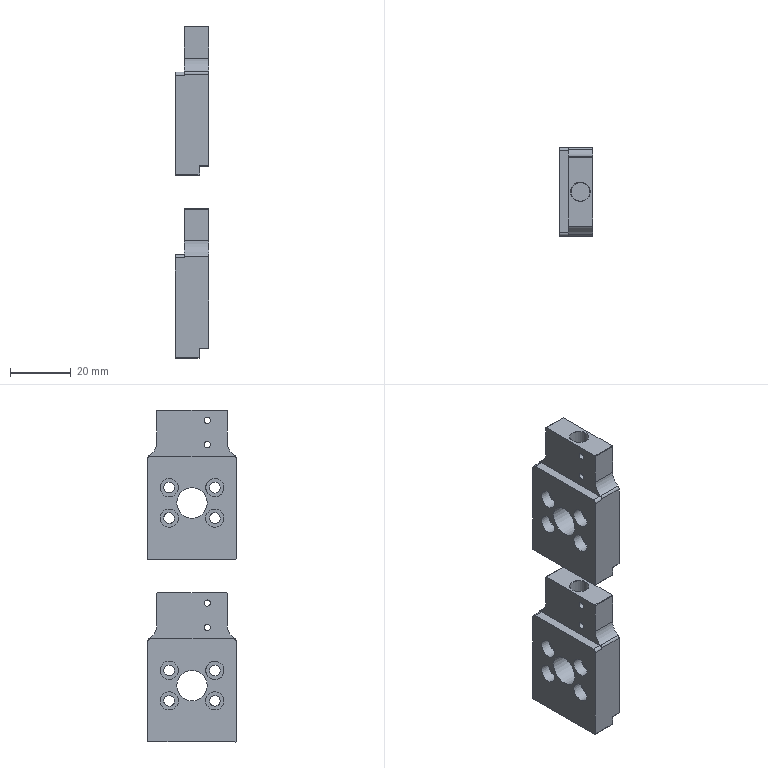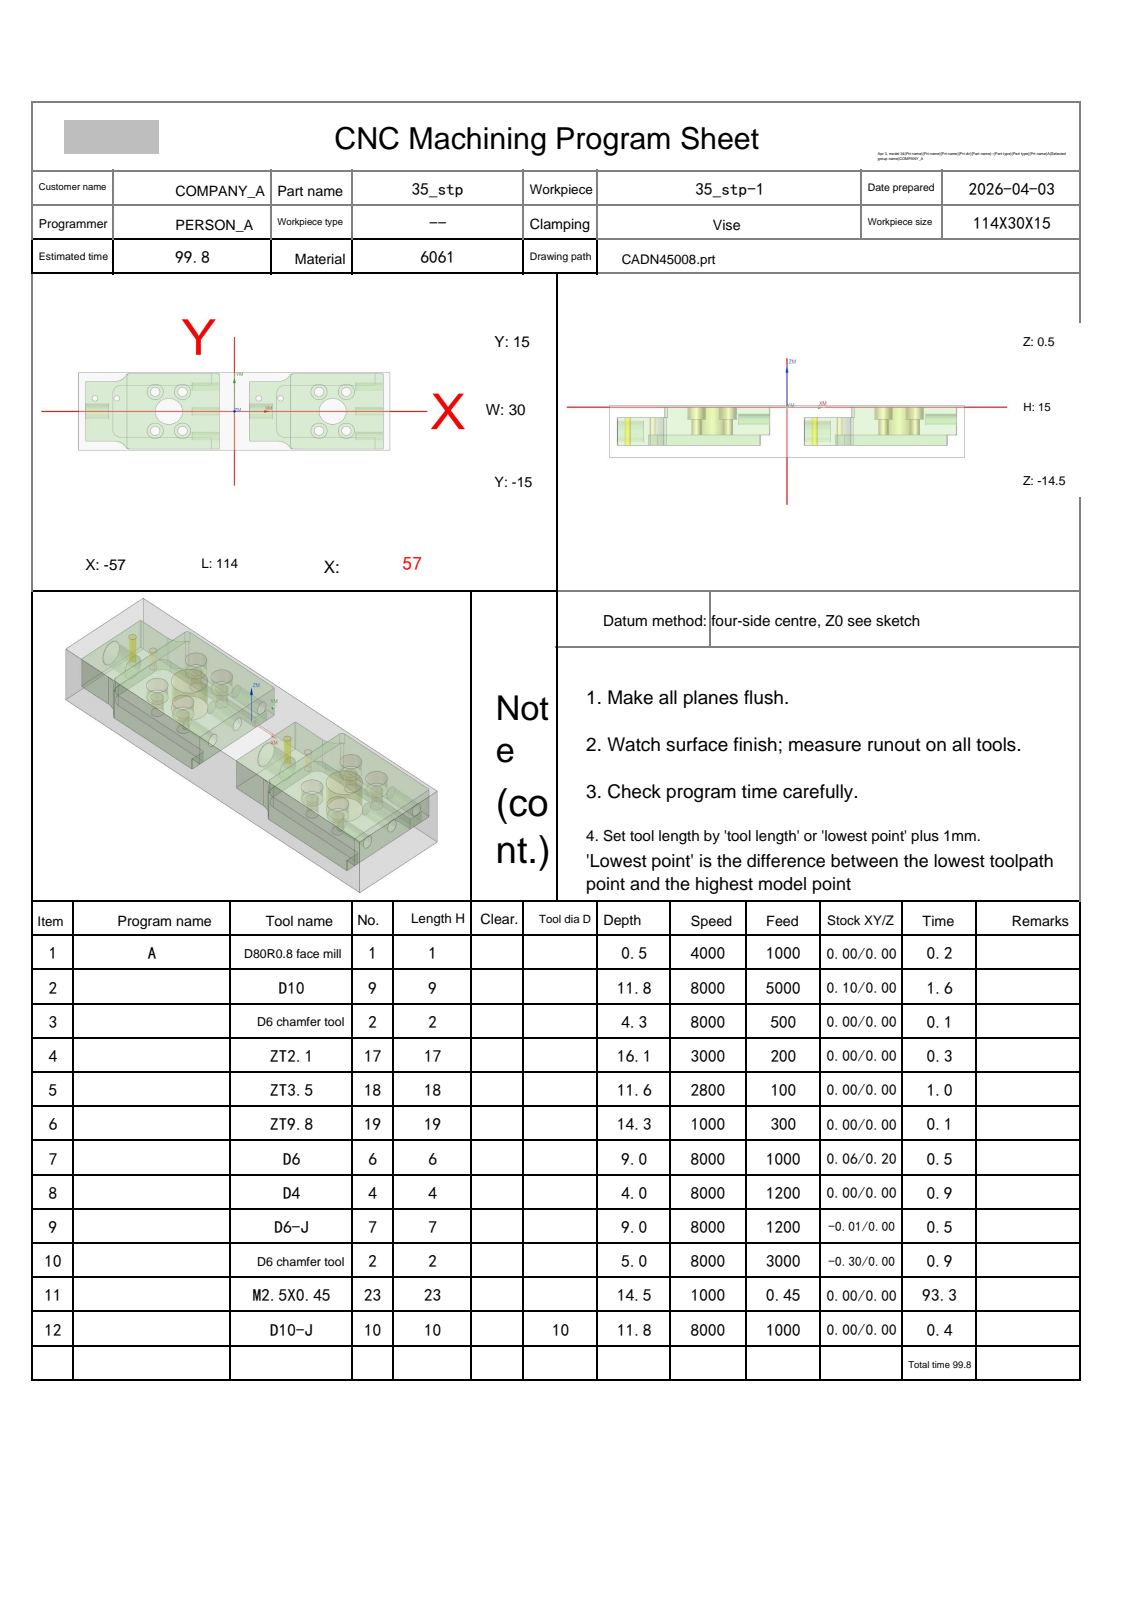NC program | NX | posted by the shop | part box 11 x 29 x 109 mm
Whole program, first 1540 of 2088 lines:
%
O0001
(Machine time: 186.62 MIN)
(===Total Tool:11===)
(T1=D80R0.8 face mill D=80.  R=0.8  D-  H01 Z=0.    )
(T9=D10     D=10.  R=0.   D-  H09 Z=-11.3 )
(T2=D6 chamfer tool   D=6.   R=0.   D-  H02 Z=-4.5  )
(T17=ZT2.1  D=2.1  DR_a=118 D-  H17 Z=-15.63)
(T18=ZT3.5  D=3.5  DR_a=118 D-  H18 Z=-11.05)
(T19=ZT9.8  D=9.8  DR_a=120 D-  H19 Z=-13.83)
(T6=D6      D=6.   R=0.   D-  H06 Z=-8.5  )
(T4=D4      D=4.   R=0.   D4  H04 Z=-3.5  )
(T7=D6-J    D=6.   R=0.   D7  H07 Z=-8.5  )
(T23=M2.5X0.45 D=2.05 DR_a=180 D-  H23 Z=-14.  )
(T10=D10-J  D=10.  R=0.   D10 H10 Z=-11.3 )
G80 G90 G17 G49 G40
G91 G28 Z0
M01
N1 T01 M06
(D80R0.8 face mill  D=80. R=0.8 H=01 ce=0.00 di=0.00)
G00 G90 G54 X99.5 Y0.0 M03 S4000
G43 H01 Z20.
M08
Z2.
G01 Z0.0 F1000.
X94.5
X-94.5
X-99.5
Z2.
G00 Z20.
G91 G28 Z0.0
M05
M09
G91 G28 Z0.0
M01
N2 T09 M06
(D10  D=10. R=0. H=09 ce=0.10 di=0.00)
G00 G90 G54 X-22.118 Y-19.6 M03 S8000
G43 H09 Z20.
M08
Z.5
G01 X-38.736 Z.429 F5000.
G02 X-43.99 Y-16.6 Z.402 I0.0 J6.1
G01 X-54.3 Z.358
G02 X-57.906 Y-15.106 Z.341 I0.0 J5.1
G01 X-58.106 Y-14.906 Z.339
G02 X-59.6 Y-11.3 Z.322 I3.606 J3.606
G01 Y11.3 Z.225
G02 X-58.106 Y14.906 Z.208 I5.1 J0.0
G01 X-57.906 Y15.106 Z.207
G02 X-54.3 Y16.6 Z.19 I3.606 J-3.606
G01 X-43.99 Z.146
G02 X-42.727 Y18.114 Z.137 I5.254 J-3.1
X-38.736 Y19.6 Z.119 I3.99 J-4.614
G01 X-5.7 Z-.023
G02 X-2.094 Y18.106 Z-.04 I0.0 J-5.1
G01 X-1.894 Y17.906 Z-.041
G02 X-.4 Y14.3 Z-.058 I-3.606 J-3.606
G01 Y-14.5 Z-.181
G02 X-5.5 Y-19.6 Z-.216 I-5.1 J0.0
G01 X-38.736 Z-.358
G02 X-43.99 Y-16.6 Z-.385 I0.0 J6.1
G01 X-54.3 Z-.429
G02 X-57.906 Y-15.106 Z-.446 I0.0 J5.1
G01 X-58.106 Y-14.906 Z-.447
G02 X-59.6 Y-11.3 Z-.464 I3.606 J3.606
G01 Y11.3 Z-.561
G02 X-58.106 Y14.906 Z-.578 I5.1 J0.0
G01 X-57.906 Y15.106 Z-.58
G02 X-54.3 Y16.6 Z-.597 I3.606 J-3.606
G01 X-43.99 Z-.641
G02 X-42.727 Y18.114 Z-.649 I5.254 J-3.1
X-38.736 Y19.6 Z-.668 I3.99 J-4.614
G01 X-5.7 Z-.809
G02 X-2.094 Y18.106 Z-.826 I0.0 J-5.1
G01 X-1.894 Y17.906 Z-.828
G02 X-.4 Y14.3 Z-.845 I-3.606 J-3.606
G01 Y-14.5 Z-.968
G02 X-5.5 Y-19.6 Z-1.002 I-5.1 J0.0
G01 X-38.736 Z-1.144
G02 X-43.99 Y-16.6 Z-1.172 I0.0 J6.1
G01 X-54.3 Z-1.216
G02 X-57.906 Y-15.106 Z-1.233 I0.0 J5.1
G01 X-58.106 Y-14.906 Z-1.234
G02 X-59.6 Y-11.3 Z-1.251 I3.606 J3.606
G01 Y11.3 Z-1.348
G02 X-58.106 Y14.906 Z-1.365 I5.1 J0.0
G01 X-57.906 Y15.106 Z-1.366
G02 X-54.3 Y16.6 Z-1.383 I3.606 J-3.606
G01 X-43.99 Z-1.427
G02 X-42.727 Y18.114 Z-1.436 I5.254 J-3.1
X-38.736 Y19.6 Z-1.455 I3.99 J-4.614
G01 X-5.7 Z-1.596
G02 X-2.094 Y18.106 Z-1.613 I0.0 J-5.1
G01 X-1.894 Y17.906 Z-1.614
G02 X-.4 Y14.3 Z-1.631 I-3.606 J-3.606
G01 Y-14.5 Z-1.755
G02 X-5.5 Y-19.6 Z-1.789 I-5.1 J0.0
G01 X-38.736 Z-1.931
G02 X-43.99 Y-16.6 Z-1.958 I0.0 J6.1
G01 X-54.3 Z-2.002
G02 X-57.906 Y-15.106 Z-2.019 I0.0 J5.1
G01 X-58.106 Y-14.906 Z-2.021
G02 X-59.6 Y-11.3 Z-2.038 I3.606 J3.606
G01 Y11.3 Z-2.135
G02 X-58.106 Y14.906 Z-2.152 I5.1 J0.0
G01 X-57.906 Y15.106 Z-2.153
G02 X-54.3 Y16.6 Z-2.17 I3.606 J-3.606
G01 X-43.99 Z-2.214
G02 X-42.727 Y18.114 Z-2.223 I5.254 J-3.1
X-38.736 Y19.6 Z-2.241 I3.99 J-4.614
G01 X-5.7 Z-2.383
G02 X-2.094 Y18.106 Z-2.4 I0.0 J-5.1
G01 X-1.894 Y17.906 Z-2.401
G02 X-.4 Y14.3 Z-2.418 I-3.606 J-3.606
G01 Y-14.5 Z-2.541
G02 X-5.5 Y-19.6 Z-2.576 I-5.1 J0.0
G01 X-38.736 Z-2.718
G02 X-43.99 Y-16.6 Z-2.745 I0.0 J6.1
G01 X-54.3 Z-2.789
G02 X-57.906 Y-15.106 Z-2.806 I0.0 J5.1
G01 X-58.106 Y-14.906 Z-2.807
G02 X-59.6 Y-11.3 Z-2.824 I3.606 J3.606
G01 Y11.3 Z-2.921
G02 X-58.106 Y14.906 Z-2.938 I5.1 J0.0
G01 X-57.906 Y15.106 Z-2.94
G02 X-54.3 Y16.6 Z-2.957 I3.606 J-3.606
G01 X-43.99 Z-3.001
G02 X-42.727 Y18.114 Z-3.009 I5.254 J-3.1
X-38.736 Y19.6 Z-3.028 I3.99 J-4.614
G01 X-5.7 Z-3.169
G02 X-2.094 Y18.106 Z-3.186 I0.0 J-5.1
G01 X-1.894 Y17.906 Z-3.188
G02 X-.4 Y14.3 Z-3.205 I-3.606 J-3.606
G01 Y-14.5 Z-3.328
G02 X-5.5 Y-19.6 Z-3.362 I-5.1 J0.0
G01 X-38.736 Z-3.504
G02 X-43.99 Y-16.6 Z-3.532 I0.0 J6.1
G01 X-54.3 Z-3.576
G02 X-57.906 Y-15.106 Z-3.593 I0.0 J5.1
G01 X-58.106 Y-14.906 Z-3.594
G02 X-59.6 Y-11.3 Z-3.611 I3.606 J3.606
G01 Y11.3 Z-3.708
G02 X-58.106 Y14.906 Z-3.725 I5.1 J0.0
G01 X-57.906 Y15.106 Z-3.726
G02 X-54.3 Y16.6 Z-3.743 I3.606 J-3.606
G01 X-43.99 Z-3.787
G02 X-42.727 Y18.114 Z-3.796 I5.254 J-3.1
X-38.736 Y19.6 Z-3.815 I3.99 J-4.614
G01 X-5.7 Z-3.956
G02 X-2.094 Y18.106 Z-3.973 I0.0 J-5.1
G01 X-1.894 Y17.906 Z-3.974
G02 X-.4 Y14.3 Z-3.991 I-3.606 J-3.606
G01 Y-14.5 Z-4.115
G02 X-5.5 Y-19.6 Z-4.149 I-5.1 J0.0
G01 X-38.736 Z-4.291
G02 X-43.99 Y-16.6 Z-4.318 I0.0 J6.1
G01 X-54.3 Z-4.362
G02 X-57.906 Y-15.106 Z-4.379 I0.0 J5.1
G01 X-58.106 Y-14.906 Z-4.381
G02 X-59.6 Y-11.3 Z-4.398 I3.606 J3.606
G01 Y11.3 Z-4.495
G02 X-58.106 Y14.906 Z-4.512 I5.1 J0.0
G01 X-57.906 Y15.106 Z-4.513
G02 X-54.3 Y16.6 Z-4.53 I3.606 J-3.606
G01 X-43.99 Z-4.574
G02 X-42.727 Y18.114 Z-4.583 I5.254 J-3.1
X-38.736 Y19.6 Z-4.601 I3.99 J-4.614
G01 X-5.7 Z-4.743
G02 X-2.094 Y18.106 Z-4.76 I0.0 J-5.1
G01 X-1.894 Y17.906 Z-4.761
G02 X-.4 Y14.3 Z-4.778 I-3.606 J-3.606
G01 Y-14.5 Z-4.901
G02 X-5.5 Y-19.6 Z-4.936 I-5.1 J0.0
G01 X-38.736 Z-5.078
G02 X-43.99 Y-16.6 Z-5.105 I0.0 J6.1
G01 X-54.3 Z-5.149
G02 X-57.906 Y-15.106 Z-5.166 I0.0 J5.1
G01 X-58.106 Y-14.906 Z-5.167
G02 X-59.6 Y-11.3 Z-5.184 I3.606 J3.606
G01 Y11.3 Z-5.281
G02 X-58.106 Y14.906 Z-5.298 I5.1 J0.0
G01 X-57.906 Y15.106 Z-5.3
G02 X-54.3 Y16.6 Z-5.317 I3.606 J-3.606
G01 X-43.99 Z-5.361
G02 X-42.727 Y18.114 Z-5.369 I5.254 J-3.1
X-38.736 Y19.6 Z-5.388 I3.99 J-4.614
G01 X-5.7 Z-5.529
G02 X-2.094 Y18.106 Z-5.546 I0.0 J-5.1
G01 X-1.894 Y17.906 Z-5.548
G02 X-.4 Y14.3 Z-5.565 I-3.606 J-3.606
G01 Y-14.5 Z-5.688
G02 X-5.5 Y-19.6 Z-5.722 I-5.1 J0.0
G01 X-38.736 Z-5.864
G02 X-43.99 Y-16.6 Z-5.892 I0.0 J6.1
G01 X-54.3 Z-5.936
G02 X-57.906 Y-15.106 Z-5.953 I0.0 J5.1
G01 X-58.106 Y-14.906 Z-5.954
G02 X-59.6 Y-11.3 Z-5.971 I3.606 J3.606
G01 Y11.3 Z-6.068
G02 X-58.106 Y14.906 Z-6.085 I5.1 J0.0
G01 X-57.906 Y15.106 Z-6.086
G02 X-54.3 Y16.6 Z-6.103 I3.606 J-3.606
G01 X-43.99 Z-6.147
G02 X-42.727 Y18.114 Z-6.156 I5.254 J-3.1
X-38.736 Y19.6 Z-6.175 I3.99 J-4.614
G01 X-5.7 Z-6.316
G02 X-2.094 Y18.106 Z-6.333 I0.0 J-5.1
G01 X-1.894 Y17.906 Z-6.334
G02 X-.4 Y14.3 Z-6.351 I-3.606 J-3.606
G01 Y-14.5 Z-6.475
G02 X-5.5 Y-19.6 Z-6.509 I-5.1 J0.0
G01 X-38.736 Z-6.651
G02 X-43.99 Y-16.6 Z-6.678 I0.0 J6.1
G01 X-54.3 Z-6.722
G02 X-57.906 Y-15.106 Z-6.739 I0.0 J5.1
G01 X-58.106 Y-14.906 Z-6.741
G02 X-59.6 Y-11.3 Z-6.758 I3.606 J3.606
G01 Y11.3 Z-6.855
G02 X-58.106 Y14.906 Z-6.872 I5.1 J0.0
G01 X-57.906 Y15.106 Z-6.873
G02 X-54.3 Y16.6 Z-6.89 I3.606 J-3.606
G01 X-43.99 Z-6.934
G02 X-42.727 Y18.114 Z-6.943 I5.254 J-3.1
X-38.736 Y19.6 Z-6.961 I3.99 J-4.614
G01 X-5.7 Z-7.103
G02 X-2.094 Y18.106 Z-7.12 I0.0 J-5.1
G01 X-1.894 Y17.906 Z-7.121
G02 X-.4 Y14.3 Z-7.138 I-3.606 J-3.606
G01 Y-14.5 Z-7.261
G02 X-5.5 Y-19.6 Z-7.296 I-5.1 J0.0
G01 X-38.736 Z-7.438
G02 X-43.99 Y-16.6 Z-7.465 I0.0 J6.1
G01 X-54.3 Z-7.509
G02 X-57.906 Y-15.106 Z-7.526 I0.0 J5.1
G01 X-58.106 Y-14.906 Z-7.527
G02 X-59.6 Y-11.3 Z-7.544 I3.606 J3.606
G01 Y11.3 Z-7.641
G02 X-58.106 Y14.906 Z-7.658 I5.1 J0.0
G01 X-57.906 Y15.106 Z-7.66
G02 X-54.3 Y16.6 Z-7.677 I3.606 J-3.606
G01 X-43.99 Z-7.721
G02 X-42.727 Y18.114 Z-7.729 I5.254 J-3.1
X-38.736 Y19.6 Z-7.748 I3.99 J-4.614
G01 X-5.7 Z-7.889
G02 X-2.094 Y18.106 Z-7.906 I0.0 J-5.1
G01 X-1.894 Y17.906 Z-7.908
G02 X-.4 Y14.3 Z-7.925 I-3.606 J-3.606
G01 Y-14.5 Z-8.048
G02 X-5.5 Y-19.6 Z-8.082 I-5.1 J0.0
G01 X-38.736 Z-8.224
G02 X-43.99 Y-16.6 Z-8.252 I0.0 J6.1
G01 X-54.3 Z-8.296
G02 X-57.906 Y-15.106 Z-8.313 I0.0 J5.1
G01 X-58.106 Y-14.906 Z-8.314
G02 X-59.6 Y-11.3 Z-8.331 I3.606 J3.606
G01 Y11.3 Z-8.428
G02 X-58.106 Y14.906 Z-8.445 I5.1 J0.0
G01 X-57.906 Y15.106 Z-8.446
G02 X-54.3 Y16.6 Z-8.463 I3.606 J-3.606
G01 X-43.99 Z-8.507
G02 X-42.727 Y18.114 Z-8.516 I5.254 J-3.1
X-38.736 Y19.6 Z-8.535 I3.99 J-4.614
G01 X-5.7 Z-8.676
G02 X-2.094 Y18.106 Z-8.693 I0.0 J-5.1
G01 X-1.894 Y17.906 Z-8.694
G02 X-.4 Y14.3 Z-8.711 I-3.606 J-3.606
G01 Y-14.5 Z-8.835
G02 X-5.5 Y-19.6 Z-8.869 I-5.1 J0.0
G01 X-38.736 Z-9.011
G02 X-43.99 Y-16.6 Z-9.038 I0.0 J6.1
G01 X-54.3 Z-9.082
G02 X-57.906 Y-15.106 Z-9.099 I0.0 J5.1
G01 X-58.106 Y-14.906 Z-9.101
G02 X-59.6 Y-11.3 Z-9.118 I3.606 J3.606
G01 Y11.3 Z-9.215
G02 X-58.106 Y14.906 Z-9.232 I5.1 J0.0
G01 X-57.906 Y15.106 Z-9.233
G02 X-54.3 Y16.6 Z-9.25 I3.606 J-3.606
G01 X-43.99 Z-9.294
G02 X-42.727 Y18.114 Z-9.303 I5.254 J-3.1
X-38.736 Y19.6 Z-9.321 I3.99 J-4.614
G01 X-5.7 Z-9.463
G02 X-2.094 Y18.106 Z-9.48 I0.0 J-5.1
G01 X-1.894 Y17.906 Z-9.481
G02 X-.4 Y14.3 Z-9.498 I-3.606 J-3.606
G01 Y-14.5 Z-9.621
G02 X-5.5 Y-19.6 Z-9.656 I-5.1 J0.0
G01 X-38.736 Z-9.798
G02 X-43.99 Y-16.6 Z-9.825 I0.0 J6.1
G01 X-54.3 Z-9.869
G02 X-57.906 Y-15.106 Z-9.886 I0.0 J5.1
G01 X-58.106 Y-14.906 Z-9.887
G02 X-59.6 Y-11.3 Z-9.904 I3.606 J3.606
G01 Y11.3 Z-10.001
G02 X-58.106 Y14.906 Z-10.018 I5.1 J0.0
G01 X-57.906 Y15.106 Z-10.02
G02 X-54.3 Y16.6 Z-10.037 I3.606 J-3.606
G01 X-43.99 Z-10.081
G02 X-42.727 Y18.114 Z-10.089 I5.254 J-3.1
X-38.736 Y19.6 Z-10.108 I3.99 J-4.614
G01 X-5.7 Z-10.249
G02 X-2.094 Y18.106 Z-10.266 I0.0 J-5.1
G01 X-1.894 Y17.906 Z-10.268
G02 X-.4 Y14.3 Z-10.285 I-3.606 J-3.606
G01 Y-14.5 Z-10.408
G02 X-5.5 Y-19.6 Z-10.442 I-5.1 J0.0
G01 X-38.736 Z-10.584
G02 X-43.99 Y-16.6 Z-10.612 I0.0 J6.1
G01 X-54.3 Z-10.656
G02 X-57.906 Y-15.106 Z-10.673 I0.0 J5.1
G01 X-58.106 Y-14.906 Z-10.674
G02 X-59.6 Y-11.3 Z-10.691 I3.606 J3.606
G01 Y11.3 Z-10.788
G02 X-58.106 Y14.906 Z-10.805 I5.1 J0.0
G01 X-57.906 Y15.106 Z-10.806
G02 X-54.3 Y16.6 Z-10.823 I3.606 J-3.606
G01 X-43.99 Z-10.867
G02 X-42.727 Y18.114 Z-10.876 I5.254 J-3.1
X-38.736 Y19.6 Z-10.895 I3.99 J-4.614
G01 X-5.7 Z-11.036
G02 X-2.094 Y18.106 Z-11.053 I0.0 J-5.1
G01 X-1.894 Y17.906 Z-11.054
G02 X-.4 Y14.3 Z-11.071 I-3.606 J-3.606
G01 Y-14.5 Z-11.195
G02 X-5.5 Y-19.6 Z-11.229 I-5.1 J0.0
G01 X-22.118 Z-11.3
X-38.736
G02 X-43.99 Y-16.6 I0.0 J6.1
G01 X-54.3
G02 X-57.906 Y-15.106 I0.0 J5.1
G01 X-58.106 Y-14.906
G02 X-59.6 Y-11.3 I3.606 J3.606
G01 Y11.3
G02 X-58.106 Y14.906 I5.1 J0.0
G01 X-57.906 Y15.106
G02 X-54.3 Y16.6 I3.606 J-3.606
G01 X-43.99
G02 X-38.736 Y19.6 I5.254 J-3.1
G01 X-5.7
G02 X-2.094 Y18.106 I0.0 J-5.1
G01 X-1.894 Y17.906
G02 X-.4 Y14.3 I-3.606 J-3.606
G01 Y-14.5
G02 X-5.5 Y-19.6 I-5.1 J0.0
G01 X-22.118
X-22.618
Z-10.3
G00 Z20.
X37.882
Z.5
G01 X21.264 Z.429
G02 X16.01 Y-16.6 Z.402 I0.0 J6.1
G01 X5.7 Z.358
G02 X2.094 Y-15.106 Z.341 I0.0 J5.1
G01 X1.894 Y-14.906 Z.339
G02 X.4 Y-11.3 Z.322 I3.606 J3.606
G01 Y11.3 Z.225
G02 X1.894 Y14.906 Z.208 I5.1 J0.0
G01 X2.094 Y15.106 Z.207
G02 X5.7 Y16.6 Z.19 I3.606 J-3.606
G01 X16.01 Z.146
G02 X21.264 Y19.6 Z.119 I5.254 J-3.1
G01 X54.3 Z-.023
G02 X57.906 Y18.106 Z-.04 I0.0 J-5.1
G01 X58.106 Y17.906 Z-.041
G02 X59.6 Y14.3 Z-.058 I-3.606 J-3.606
G01 Y-14.5 Z-.181
G02 X54.5 Y-19.6 Z-.216 I-5.1 J0.0
G01 X21.264 Z-.358
G02 X16.01 Y-16.6 Z-.385 I0.0 J6.1
G01 X5.7 Z-.429
G02 X2.094 Y-15.106 Z-.446 I0.0 J5.1
G01 X1.894 Y-14.906 Z-.447
G02 X.4 Y-11.3 Z-.464 I3.606 J3.606
G01 Y11.3 Z-.561
G02 X1.894 Y14.906 Z-.578 I5.1 J0.0
G01 X2.094 Y15.106 Z-.58
G02 X5.7 Y16.6 Z-.597 I3.606 J-3.606
G01 X16.01 Z-.641
G02 X21.264 Y19.6 Z-.668 I5.254 J-3.1
G01 X54.3 Z-.809
G02 X57.906 Y18.106 Z-.826 I0.0 J-5.1
G01 X58.106 Y17.906 Z-.828
G02 X59.6 Y14.3 Z-.845 I-3.606 J-3.606
G01 Y-14.5 Z-.968
G02 X54.5 Y-19.6 Z-1.002 I-5.1 J0.0
G01 X21.264 Z-1.144
G02 X16.01 Y-16.6 Z-1.172 I0.0 J6.1
G01 X5.7 Z-1.216
G02 X2.094 Y-15.106 Z-1.233 I0.0 J5.1
G01 X1.894 Y-14.906 Z-1.234
G02 X.4 Y-11.3 Z-1.251 I3.606 J3.606
G01 Y11.3 Z-1.348
G02 X1.894 Y14.906 Z-1.365 I5.1 J0.0
G01 X2.094 Y15.106 Z-1.366
G02 X5.7 Y16.6 Z-1.383 I3.606 J-3.606
G01 X16.01 Z-1.427
G02 X21.264 Y19.6 Z-1.455 I5.254 J-3.1
G01 X54.3 Z-1.596
G02 X57.906 Y18.106 Z-1.613 I0.0 J-5.1
G01 X58.106 Y17.906 Z-1.614
G02 X59.6 Y14.3 Z-1.631 I-3.606 J-3.606
G01 Y-14.5 Z-1.755
G02 X54.5 Y-19.6 Z-1.789 I-5.1 J0.0
G01 X21.264 Z-1.931
G02 X16.01 Y-16.6 Z-1.958 I0.0 J6.1
G01 X5.7 Z-2.002
G02 X2.094 Y-15.106 Z-2.019 I0.0 J5.1
G01 X1.894 Y-14.906 Z-2.021
G02 X.4 Y-11.3 Z-2.038 I3.606 J3.606
G01 Y11.3 Z-2.135
G02 X1.894 Y14.906 Z-2.152 I5.1 J0.0
G01 X2.094 Y15.106 Z-2.153
G02 X5.7 Y16.6 Z-2.17 I3.606 J-3.606
G01 X16.01 Z-2.214
G02 X21.264 Y19.6 Z-2.241 I5.254 J-3.1
G01 X54.3 Z-2.383
G02 X57.906 Y18.106 Z-2.4 I0.0 J-5.1
G01 X58.106 Y17.906 Z-2.401
G02 X59.6 Y14.3 Z-2.418 I-3.606 J-3.606
G01 Y-14.5 Z-2.541
G02 X54.5 Y-19.6 Z-2.576 I-5.1 J0.0
G01 X21.264 Z-2.718
G02 X16.01 Y-16.6 Z-2.745 I0.0 J6.1
G01 X5.7 Z-2.789
G02 X2.094 Y-15.106 Z-2.806 I0.0 J5.1
G01 X1.894 Y-14.906 Z-2.807
G02 X.4 Y-11.3 Z-2.824 I3.606 J3.606
G01 Y11.3 Z-2.921
G02 X1.894 Y14.906 Z-2.938 I5.1 J0.0
G01 X2.094 Y15.106 Z-2.94
G02 X5.7 Y16.6 Z-2.957 I3.606 J-3.606
G01 X16.01 Z-3.001
G02 X21.264 Y19.6 Z-3.028 I5.254 J-3.1
G01 X54.3 Z-3.169
G02 X57.906 Y18.106 Z-3.186 I0.0 J-5.1
G01 X58.106 Y17.906 Z-3.188
G02 X59.6 Y14.3 Z-3.205 I-3.606 J-3.606
G01 Y-14.5 Z-3.328
G02 X54.5 Y-19.6 Z-3.362 I-5.1 J0.0
G01 X21.264 Z-3.504
G02 X16.01 Y-16.6 Z-3.532 I0.0 J6.1
G01 X5.7 Z-3.576
G02 X2.094 Y-15.106 Z-3.593 I0.0 J5.1
G01 X1.894 Y-14.906 Z-3.594
G02 X.4 Y-11.3 Z-3.611 I3.606 J3.606
G01 Y11.3 Z-3.708
G02 X1.894 Y14.906 Z-3.725 I5.1 J0.0
G01 X2.094 Y15.106 Z-3.726
G02 X5.7 Y16.6 Z-3.743 I3.606 J-3.606
G01 X16.01 Z-3.787
G02 X21.264 Y19.6 Z-3.815 I5.254 J-3.1
G01 X54.3 Z-3.956
G02 X57.906 Y18.106 Z-3.973 I0.0 J-5.1
G01 X58.106 Y17.906 Z-3.974
G02 X59.6 Y14.3 Z-3.991 I-3.606 J-3.606
G01 Y-14.5 Z-4.115
G02 X54.5 Y-19.6 Z-4.149 I-5.1 J0.0
G01 X21.264 Z-4.291
G02 X16.01 Y-16.6 Z-4.318 I0.0 J6.1
G01 X5.7 Z-4.362
G02 X2.094 Y-15.106 Z-4.379 I0.0 J5.1
G01 X1.894 Y-14.906 Z-4.381
G02 X.4 Y-11.3 Z-4.398 I3.606 J3.606
G01 Y11.3 Z-4.495
G02 X1.894 Y14.906 Z-4.512 I5.1 J0.0
G01 X2.094 Y15.106 Z-4.513
G02 X5.7 Y16.6 Z-4.53 I3.606 J-3.606
G01 X16.01 Z-4.574
G02 X21.264 Y19.6 Z-4.601 I5.254 J-3.1
G01 X54.3 Z-4.743
G02 X57.906 Y18.106 Z-4.76 I0.0 J-5.1
G01 X58.106 Y17.906 Z-4.761
G02 X59.6 Y14.3 Z-4.778 I-3.606 J-3.606
G01 Y-14.5 Z-4.901
G02 X54.5 Y-19.6 Z-4.936 I-5.1 J0.0
G01 X21.264 Z-5.078
G02 X16.01 Y-16.6 Z-5.105 I0.0 J6.1
G01 X5.7 Z-5.149
G02 X2.094 Y-15.106 Z-5.166 I0.0 J5.1
G01 X1.894 Y-14.906 Z-5.167
G02 X.4 Y-11.3 Z-5.184 I3.606 J3.606
G01 Y11.3 Z-5.281
G02 X1.894 Y14.906 Z-5.298 I5.1 J0.0
G01 X2.094 Y15.106 Z-5.3
G02 X5.7 Y16.6 Z-5.317 I3.606 J-3.606
G01 X16.01 Z-5.361
G02 X21.264 Y19.6 Z-5.388 I5.254 J-3.1
G01 X54.3 Z-5.529
G02 X57.906 Y18.106 Z-5.546 I0.0 J-5.1
G01 X58.106 Y17.906 Z-5.548
G02 X59.6 Y14.3 Z-5.565 I-3.606 J-3.606
G01 Y-14.5 Z-5.688
G02 X54.5 Y-19.6 Z-5.722 I-5.1 J0.0
G01 X21.264 Z-5.864
G02 X16.01 Y-16.6 Z-5.892 I0.0 J6.1
G01 X5.7 Z-5.936
G02 X2.094 Y-15.106 Z-5.953 I0.0 J5.1
G01 X1.894 Y-14.906 Z-5.954
G02 X.4 Y-11.3 Z-5.971 I3.606 J3.606
G01 Y11.3 Z-6.068
G02 X1.894 Y14.906 Z-6.085 I5.1 J0.0
G01 X2.094 Y15.106 Z-6.086
G02 X5.7 Y16.6 Z-6.103 I3.606 J-3.606
G01 X16.01 Z-6.147
G02 X21.264 Y19.6 Z-6.175 I5.254 J-3.1
G01 X54.3 Z-6.316
G02 X57.906 Y18.106 Z-6.333 I0.0 J-5.1
G01 X58.106 Y17.906 Z-6.334
G02 X59.6 Y14.3 Z-6.351 I-3.606 J-3.606
G01 Y-14.5 Z-6.475
G02 X54.5 Y-19.6 Z-6.509 I-5.1 J0.0
G01 X21.264 Z-6.651
G02 X16.01 Y-16.6 Z-6.678 I0.0 J6.1
G01 X5.7 Z-6.722
G02 X2.094 Y-15.106 Z-6.739 I0.0 J5.1
G01 X1.894 Y-14.906 Z-6.741
G02 X.4 Y-11.3 Z-6.758 I3.606 J3.606
G01 Y11.3 Z-6.855
G02 X1.894 Y14.906 Z-6.872 I5.1 J0.0
G01 X2.094 Y15.106 Z-6.873
G02 X5.7 Y16.6 Z-6.89 I3.606 J-3.606
G01 X16.01 Z-6.934
G02 X21.264 Y19.6 Z-6.961 I5.254 J-3.1
G01 X54.3 Z-7.103
G02 X57.906 Y18.106 Z-7.12 I0.0 J-5.1
G01 X58.106 Y17.906 Z-7.121
G02 X59.6 Y14.3 Z-7.138 I-3.606 J-3.606
G01 Y-14.5 Z-7.261
G02 X54.5 Y-19.6 Z-7.296 I-5.1 J0.0
G01 X21.264 Z-7.438
G02 X16.01 Y-16.6 Z-7.465 I0.0 J6.1
G01 X5.7 Z-7.509
G02 X2.094 Y-15.106 Z-7.526 I0.0 J5.1
G01 X1.894 Y-14.906 Z-7.527
G02 X.4 Y-11.3 Z-7.544 I3.606 J3.606
G01 Y11.3 Z-7.641
G02 X1.894 Y14.906 Z-7.658 I5.1 J0.0
G01 X2.094 Y15.106 Z-7.66
G02 X5.7 Y16.6 Z-7.677 I3.606 J-3.606
G01 X16.01 Z-7.721
G02 X21.264 Y19.6 Z-7.748 I5.254 J-3.1
G01 X54.3 Z-7.889
G02 X57.906 Y18.106 Z-7.906 I0.0 J-5.1
G01 X58.106 Y17.906 Z-7.908
G02 X59.6 Y14.3 Z-7.925 I-3.606 J-3.606
G01 Y-14.5 Z-8.048
G02 X54.5 Y-19.6 Z-8.082 I-5.1 J0.0
G01 X21.264 Z-8.224
G02 X16.01 Y-16.6 Z-8.252 I0.0 J6.1
G01 X5.7 Z-8.296
G02 X2.094 Y-15.106 Z-8.313 I0.0 J5.1
G01 X1.894 Y-14.906 Z-8.314
G02 X.4 Y-11.3 Z-8.331 I3.606 J3.606
G01 Y11.3 Z-8.428
G02 X1.894 Y14.906 Z-8.445 I5.1 J0.0
G01 X2.094 Y15.106 Z-8.446
G02 X5.7 Y16.6 Z-8.463 I3.606 J-3.606
G01 X16.01 Z-8.507
G02 X21.264 Y19.6 Z-8.535 I5.254 J-3.1
G01 X54.3 Z-8.676
G02 X57.906 Y18.106 Z-8.693 I0.0 J-5.1
G01 X58.106 Y17.906 Z-8.694
G02 X59.6 Y14.3 Z-8.711 I-3.606 J-3.606
G01 Y-14.5 Z-8.835
G02 X54.5 Y-19.6 Z-8.869 I-5.1 J0.0
G01 X21.264 Z-9.011
G02 X16.01 Y-16.6 Z-9.038 I0.0 J6.1
G01 X5.7 Z-9.082
G02 X2.094 Y-15.106 Z-9.099 I0.0 J5.1
G01 X1.894 Y-14.906 Z-9.101
G02 X.4 Y-11.3 Z-9.118 I3.606 J3.606
G01 Y11.3 Z-9.215
G02 X1.894 Y14.906 Z-9.232 I5.1 J0.0
G01 X2.094 Y15.106 Z-9.233
G02 X5.7 Y16.6 Z-9.25 I3.606 J-3.606
G01 X16.01 Z-9.294
G02 X21.264 Y19.6 Z-9.321 I5.254 J-3.1
G01 X54.3 Z-9.463
G02 X57.906 Y18.106 Z-9.48 I0.0 J-5.1
G01 X58.106 Y17.906 Z-9.481
G02 X59.6 Y14.3 Z-9.498 I-3.606 J-3.606
G01 Y-14.5 Z-9.621
G02 X54.5 Y-19.6 Z-9.656 I-5.1 J0.0
G01 X21.264 Z-9.798
G02 X16.01 Y-16.6 Z-9.825 I0.0 J6.1
G01 X5.7 Z-9.869
G02 X2.094 Y-15.106 Z-9.886 I0.0 J5.1
G01 X1.894 Y-14.906 Z-9.887
G02 X.4 Y-11.3 Z-9.904 I3.606 J3.606
G01 Y11.3 Z-10.001
G02 X1.894 Y14.906 Z-10.018 I5.1 J0.0
G01 X2.094 Y15.106 Z-10.02
G02 X5.7 Y16.6 Z-10.037 I3.606 J-3.606
G01 X16.01 Z-10.081
G02 X21.264 Y19.6 Z-10.108 I5.254 J-3.1
G01 X54.3 Z-10.249
G02 X57.906 Y18.106 Z-10.266 I0.0 J-5.1
G01 X58.106 Y17.906 Z-10.268
G02 X59.6 Y14.3 Z-10.285 I-3.606 J-3.606
G01 Y-14.5 Z-10.408
G02 X54.5 Y-19.6 Z-10.442 I-5.1 J0.0
G01 X21.264 Z-10.584
G02 X16.01 Y-16.6 Z-10.612 I0.0 J6.1
G01 X5.7 Z-10.656
G02 X2.094 Y-15.106 Z-10.673 I0.0 J5.1
G01 X1.894 Y-14.906 Z-10.674
G02 X.4 Y-11.3 Z-10.691 I3.606 J3.606
G01 Y11.3 Z-10.788
G02 X1.894 Y14.906 Z-10.805 I5.1 J0.0
G01 X2.094 Y15.106 Z-10.806
G02 X5.7 Y16.6 Z-10.823 I3.606 J-3.606
G01 X16.01 Z-10.867
G02 X21.264 Y19.6 Z-10.895 I5.254 J-3.1
G01 X54.3 Z-11.036
G02 X57.906 Y18.106 Z-11.053 I0.0 J-5.1
G01 X58.106 Y17.906 Z-11.054
G02 X59.6 Y14.3 Z-11.071 I-3.606 J-3.606
G01 Y-14.5 Z-11.195
G02 X54.5 Y-19.6 Z-11.229 I-5.1 J0.0
G01 X37.882 Z-11.3
X21.264
G02 X16.01 Y-16.6 I0.0 J6.1
G01 X5.7
G02 X2.094 Y-15.106 I0.0 J5.1
G01 X1.894 Y-14.906
G02 X.4 Y-11.3 I3.606 J3.606
G01 Y11.3
G02 X1.894 Y14.906 I5.1 J0.0
G01 X2.094 Y15.106
G02 X5.7 Y16.6 I3.606 J-3.606
G01 X16.01
G02 X21.264 Y19.6 I5.254 J-3.1
G01 X54.3
G02 X57.906 Y18.106 I0.0 J-5.1
G01 X58.106 Y17.906
G02 X59.6 Y14.3 I-3.606 J-3.606
G01 Y-14.5
G02 X54.5 Y-19.6 I-5.1 J0.0
G01 X37.882
X37.382
Z-10.3
G00 Z20.
G00 G90 X10.025 Y-19.5 M03 S6000
Z20.
Z.017
G01 Z-.483 F3500.
Y-8.
X11.05
Y8.
X9.
Y-8.
X10.025
Y-12.5
X15.55
Y12.5
X5.286
X4.5 Y11.714
Y-11.714
X5.286 Y-12.5
X10.025
X10.525
Z.017
G00 Z.5
X10.025 Y-19.5
Z-.467
G01 Z-.967
Y-8.
X11.05
Y8.
X9.
Y-8.
X10.025
Y-12.5
X15.55
Y12.5
X5.286
X4.5 Y11.714
Y-11.714
X5.286 Y-12.5
X10.025
X10.525
Z-.467
G00 Z.017
X10.025 Y-19.5
Z-.95
G01 Z-1.45
Y-8.
X11.05
Y8.
X9.
Y-8.
X10.025
Y-12.5
X15.55
Y12.5
X5.286
X4.5 Y11.714
Y-11.714
X5.286 Y-12.5
X10.025
X10.525
Z-.95
G00 Z-.467
X10.025 Y-19.5
Z-1.433
G01 Z-1.933
Y-8.
X11.05
Y8.
X9.
Y-8.
X10.025
Y-12.5
X15.55
Y12.5
X5.286
X4.5 Y11.714
Y-11.714
X5.286 Y-12.5
X10.025
X10.525
Z-1.433
G00 Z-.95
X10.025 Y-19.5
Z-1.917
G01 Z-2.417
Y-8.
X11.05
Y8.
X9.
Y-8.
X10.025
Y-12.5
X15.55
Y12.5
X5.286
X4.5 Y11.714
Y-11.714
X5.286 Y-12.5
X10.025
X10.525
Z-1.917
G00 Z-1.433
X10.025 Y-19.5
Z-2.4
G01 Z-2.9
Y-8.
X11.05
Y8.
X9.
Y-8.
X10.025
Y-12.5
X15.55
Y12.5
X5.286
X4.5 Y11.714
Y-11.714
X5.286 Y-12.5
X10.025
X10.525
Z-2.4
G00 Z20.
X-62.5 Y0.0
Z.017
G01 Z-.483
X-51.
Y-8.
X-48.95
Y8.
X-51.
Y0.0
X-55.5
Y-11.714
X-54.714 Y-12.5
X-44.45
Y12.5
X-54.714
X-55.5 Y11.714
Y0.0
Y-.5
Z.017
G00 Z.5
X-62.5 Y0.0
Z-.467
G01 Z-.967
X-51.
Y-8.
X-48.95
Y8.
X-51.
Y0.0
X-55.5
Y-11.714
X-54.714 Y-12.5
X-44.45
Y12.5
X-54.714
X-55.5 Y11.714
Y0.0
Y-.5
Z-.467
G00 Z.017
X-62.5 Y0.0
Z-.95
G01 Z-1.45
X-51.
Y-8.
X-48.95
Y8.
X-51.
Y0.0
X-55.5
Y-11.714
X-54.714 Y-12.5
X-44.45
Y12.5
X-54.714
X-55.5 Y11.714
Y0.0
Y-.5
Z-.95
G00 Z-.467
X-62.5 Y0.0
Z-1.433
G01 Z-1.933
X-51.
Y-8.
X-48.95
Y8.
X-51.
Y0.0
X-55.5
Y-11.714
X-54.714 Y-12.5
X-44.45
Y12.5
X-54.714
X-55.5 Y11.714
Y0.0
Y-.5
Z-1.433
G00 Z-.95
X-62.5 Y0.0
Z-1.917
G01 Z-2.417
X-51.
Y-8.
X-48.95
Y8.
X-51.
Y0.0
X-55.5
Y-11.714
X-54.714 Y-12.5
X-44.45
Y12.5
X-54.714
X-55.5 Y11.714
Y0.0
Y-.5
Z-1.917
G00 Z-1.433
X-62.5 Y0.0
Z-2.4
G01 Z-2.9
X-51.
Y-8.
X-48.95
Y8.
X-51.
Y0.0
X-55.5
Y-11.714
X-54.714 Y-12.5
X-44.45
Y12.5
X-54.714
X-55.5 Y11.714
Y0.0
Y-.5
Z-2.4
G00 Z20.
G91 G28 Z0.0
M05
M09
G91 G28 Z0.0
M01
N3 T02 M06
(D6 chamfer tool  D=6. R=0. H=02 ce=0.00 di=0.10)
G00 G90 G54 X-51.1 Y5. M03 S8000
G43 H02 Z20.
M08
G98 G81 X-51.1 Y5. Z-3.8 R-2. F500.
X-43.1
X-29. Y7.5 Z-.8 R1.
X-19.
X-24. Y0.0
X-29. Y-7.5
X-19.
X8.9 Y5. Z-3.8 R-2.
X16.9
X31. Y7.5 Z-.8 R1.
X41.
X36. Y0.0
X41. Y-7.5
X31.
G80
G00 Z20.
G00 G90 X-51.1 Y5. M03 S8000
Z20.
G98 G81 X-51.1 Y5. Z-3.8 R-2. F500.
X-43.1
X8.9
X16.9
G80
G00 Z20.
G91 G28 Z0.0
M05
M09
G91 G28 Z0.0
M01
N4 T17 M06
(ZT2.1 D=2.1 DR_a=118 H=17)
G00 G90 G54 X-51.1 Y5. M03 S3000
G43 H17 Z20.
M08
G98 G83 X-51.1 Y5. Z-15.631 R-2. F200. Q2.
G98 G83 X-43.1 Y5. Z-12.631 R-2. Q2.
G98 G83 X8.9 Y5. Z-15.631 R-2. Q2.
G98 G83 X16.9 Y5. Z-12.631 R-2. Q2.
G80
G00 Z20.
G91 G28 Z0.0
M05
M09
G91 G28 Z0.0
M01
N5 T18 M06
(ZT3.5 D=3.5 DR_a=118 H=18)
G00 G90 G54 X-19. Y7.5 M03 S2800
G43 H18 Z20.
M08
G98 G83 X-19. Y7.5 Z-11.052 R1. F100. Q2.
X-29.
Y-7.5
X-19.
X31.
X41.
Y7.5
X31.
G80
G00 Z20.
G91 G28 Z0.0
M05
M09
G91 G28 Z0.0
M01
N6 T19 M06
(ZT9.8 D=9.8 DR_a=120 H=19)
G00 G90 G54 X-24. Y0.0 M03 S1000
G43 H19 Z20.
M08
G98 G83 X-24. Y0.0 Z-13.829 R1. F300. Q2.
X36.
G80
G00 Z20.
G91 G28 Z0.0
M05
M09
G91 G28 Z0.0
M01
N7 T06 M06
(D6  D=6. R=0. H=06 ce=0.06 di=0.20)
G00 G90 G54 X-24. Y0.0 M03 S8000
G43 H06 Z20.
M08
Z.5
G03 X-24.97 Y-.97 I0.0 J-.97 F1000.
X-24. Y-1.94 I.97 J0.0
X-24. Y-1.94 Z0.0 I0.0 J1.94
X-24. Y-1.94 Z-.5 I0.0 J1.94
X-24. Y-1.94 Z-1. I0.0 J1.94
X-24. Y-1.94 Z-1.5 I0.0 J1.94
X-24. Y-1.94 Z-2. I0.0 J1.94
X-24. Y-1.94 Z-2.5 I0.0 J1.94
X-24. Y-1.94 Z-3. I0.0 J1.94
X-24. Y-1.94 Z-3.5 I0.0 J1.94
X-24. Y-1.94 Z-4. I0.0 J1.94
X-24. Y-1.94 Z-4.5 I0.0 J1.94
X-24. Y-1.94 Z-5. I0.0 J1.94
X-24. Y-1.94 Z-5.5 I0.0 J1.94
X-24. Y-1.94 Z-6. I0.0 J1.94
X-24. Y-1.94 Z-6.5 I0.0 J1.94
X-24. Y-1.94 Z-7. I0.0 J1.94
X-24. Y-1.94 Z-7.5 I0.0 J1.94
X-24. Y-1.94 Z-8. I0.0 J1.94
X-24. Y-1.94 Z-8.5 I0.0 J1.94
X-22.06 Y0.0 I0.0 J1.94
X-24. Y1.94 I-1.94 J0.0
X-25.94 Y0.0 I0.0 J-1.94
X-24. Y-1.94 I1.94 J0.0
X-23.03 Y-.97 I0.0 J.97
X-24. Y0.0 I-.97 J0.0
G00 Z20.
X36.
Z.5
G03 X35.03 Y-.97 I0.0 J-.97
X36. Y-1.94 I.97 J0.0
X36. Y-1.94 Z0.0 I0.0 J1.94
X36. Y-1.94 Z-.5 I0.0 J1.94
X36. Y-1.94 Z-1. I0.0 J1.94
X36. Y-1.94 Z-1.5 I0.0 J1.94
X36. Y-1.94 Z-2. I0.0 J1.94
X36. Y-1.94 Z-2.5 I0.0 J1.94
X36. Y-1.94 Z-3. I0.0 J1.94
X36. Y-1.94 Z-3.5 I0.0 J1.94
X36. Y-1.94 Z-4. I0.0 J1.94
X36. Y-1.94 Z-4.5 I0.0 J1.94
X36. Y-1.94 Z-5. I0.0 J1.94
X36. Y-1.94 Z-5.5 I0.0 J1.94
X36. Y-1.94 Z-6. I0.0 J1.94
X36. Y-1.94 Z-6.5 I0.0 J1.94
X36. Y-1.94 Z-7. I0.0 J1.94
X36. Y-1.94 Z-7.5 I0.0 J1.94
X36. Y-1.94 Z-8. I0.0 J1.94
X36. Y-1.94 Z-8.5 I0.0 J1.94
X37.94 Y0.0 I0.0 J1.94
X36. Y1.94 I-1.94 J0.0
X34.06 Y0.0 I0.0 J-1.94
X36. Y-1.94 I1.94 J0.0
X36.97 Y-.97 I0.0 J.97
X36. Y0.0 I-.97 J0.0
G00 Z20.
G91 G28 Z0.0
M05
M09
G91 G28 Z0.0
M01
N8 T04 M06
(D4  D=4. R=0. H=04 ce=0.10 di=0.00)
G00 G90 G54 X-19. Y-7.5 M03 S8000
G43 H04 Z20.
M08
Z.5
G03 X-19.45 Y-7.95 I0.0 J-.45 F1200.
X-19. Y-8.4 I.45 J0.0
X-19. Y-8.4 Z.2 I0.0 J.9
X-19. Y-8.4 Z-.1 I0.0 J.9
X-19. Y-8.4 Z-.4 I0.0 J.9
X-19. Y-8.4 Z-.7 I0.0 J.9
X-19. Y-8.4 Z-1. I0.0 J.9
X-19. Y-8.4 Z-1.3 I0.0 J.9
X-19. Y-8.4 Z-1.6 I0.0 J.9
X-19. Y-8.4 Z-1.9 I0.0 J.9
X-19. Y-8.4 Z-2.2 I0.0 J.9
X-19. Y-8.4 Z-2.5 I0.0 J.9
X-19. Y-8.4 Z-2.8 I0.0 J.9
X-19. Y-8.4 Z-3.1 I0.0 J.9
X-19. Y-8.4 Z-3.4 I0.0 J.9
X-18.221 Y-7.05 Z-3.5 I0.0 J.9
X-19. Y-6.6 I-.779 J-.45
X-19.9 Y-7.5 I0.0 J-.9
X-19. Y-8.4 I.9 J0.0
X-18.1 Y-7.5 I0.0 J.9
X-18.221 Y-7.05 I-.9 J0.0
X-18.61 Y-6.825 I-.39 J-.225
X-19.06 Y-7.275 I0.0 J-.45
X-19. Y-7.5 I.45 J0.0
G00 Z20.
X-29.
Z.5
G03 X-29.45 Y-7.95 I0.0 J-.45
X-29. Y-8.4 I.45 J0.0
X-29. Y-8.4 Z.2 I0.0 J.9
X-29. Y-8.4 Z-.1 I0.0 J.9
X-29. Y-8.4 Z-.4 I0.0 J.9
X-29. Y-8.4 Z-.7 I0.0 J.9
X-29. Y-8.4 Z-1. I0.0 J.9
X-29. Y-8.4 Z-1.3 I0.0 J.9
X-29. Y-8.4 Z-1.6 I0.0 J.9
X-29. Y-8.4 Z-1.9 I0.0 J.9
X-29. Y-8.4 Z-2.2 I0.0 J.9
X-29. Y-8.4 Z-2.5 I0.0 J.9
X-29. Y-8.4 Z-2.8 I0.0 J.9
X-29. Y-8.4 Z-3.1 I0.0 J.9
X-29. Y-8.4 Z-3.4 I0.0 J.9
X-28.221 Y-7.05 Z-3.5 I0.0 J.9
X-29. Y-6.6 I-.779 J-.45
X-29.9 Y-7.5 I0.0 J-.9
X-29. Y-8.4 I.9 J0.0
X-28.1 Y-7.5 I0.0 J.9
X-28.221 Y-7.05 I-.9 J0.0
X-28.61 Y-6.825 I-.39 J-.225
X-29.06 Y-7.275 I0.0 J-.45
X-29. Y-7.5 I.45 J0.0
G00 Z20.
Y7.5
Z.5
G03 X-29.45 Y7.05 I0.0 J-.45
X-29. Y6.6 I.45 J0.0
X-29. Y6.6 Z.2 I0.0 J.9
X-29. Y6.6 Z-.1 I0.0 J.9
X-29. Y6.6 Z-.4 I0.0 J.9
X-29. Y6.6 Z-.7 I0.0 J.9
X-29. Y6.6 Z-1. I0.0 J.9
X-29. Y6.6 Z-1.3 I0.0 J.9
X-29. Y6.6 Z-1.6 I0.0 J.9
X-29. Y6.6 Z-1.9 I0.0 J.9
X-29. Y6.6 Z-2.2 I0.0 J.9
X-29. Y6.6 Z-2.5 I0.0 J.9
X-29. Y6.6 Z-2.8 I0.0 J.9
X-29. Y6.6 Z-3.1 I0.0 J.9
X-29. Y6.6 Z-3.4 I0.0 J.9
X-28.221 Y7.95 Z-3.5 I0.0 J.9
X-29. Y8.4 I-.779 J-.45
X-29.9 Y7.5 I0.0 J-.9
X-29. Y6.6 I.9 J0.0
X-28.1 Y7.5 I0.0 J.9
X-28.221 Y7.95 I-.9 J0.0
X-28.61 Y8.175 I-.39 J-.225
X-29.06 Y7.725 I0.0 J-.45
X-29. Y7.5 I.45 J0.0
G00 Z20.
X-19.
Z.5
G03 X-19.45 Y7.05 I0.0 J-.45
X-19. Y6.6 I.45 J0.0
X-19. Y6.6 Z.2 I0.0 J.9
X-19. Y6.6 Z-.1 I0.0 J.9
X-19. Y6.6 Z-.4 I0.0 J.9
X-19. Y6.6 Z-.7 I0.0 J.9
X-19. Y6.6 Z-1. I0.0 J.9
X-19. Y6.6 Z-1.3 I0.0 J.9
X-19. Y6.6 Z-1.6 I0.0 J.9
X-19. Y6.6 Z-1.9 I0.0 J.9
X-19. Y6.6 Z-2.2 I0.0 J.9
X-19. Y6.6 Z-2.5 I0.0 J.9
X-19. Y6.6 Z-2.8 I0.0 J.9
X-19. Y6.6 Z-3.1 I0.0 J.9
X-19. Y6.6 Z-3.4 I0.0 J.9
X-18.221 Y7.95 Z-3.5 I0.0 J.9
X-19. Y8.4 I-.779 J-.45
X-19.9 Y7.5 I0.0 J-.9
X-19. Y6.6 I.9 J0.0
X-18.1 Y7.5 I0.0 J.9
X-18.221 Y7.95 I-.9 J0.0
X-18.61 Y8.175 I-.39 J-.225
X-19.06 Y7.725 I0.0 J-.45
X-19. Y7.5 I.45 J0.0
G00 Z20.
X31.
Z.5
G03 X30.55 Y7.05 I0.0 J-.45
X31. Y6.6 I.45 J0.0
X31. Y6.6 Z.2 I0.0 J.9
X31. Y6.6 Z-.1 I0.0 J.9
X31. Y6.6 Z-.4 I0.0 J.9
X31. Y6.6 Z-.7 I0.0 J.9
X31. Y6.6 Z-1. I0.0 J.9
X31. Y6.6 Z-1.3 I0.0 J.9
X31. Y6.6 Z-1.6 I0.0 J.9
X31. Y6.6 Z-1.9 I0.0 J.9
X31. Y6.6 Z-2.2 I0.0 J.9
X31. Y6.6 Z-2.5 I0.0 J.9
X31. Y6.6 Z-2.8 I0.0 J.9
X31. Y6.6 Z-3.1 I0.0 J.9
X31. Y6.6 Z-3.4 I0.0 J.9
X31.779 Y7.95 Z-3.5 I0.0 J.9
X31. Y8.4 I-.779 J-.45
X30.1 Y7.5 I0.0 J-.9
X31. Y6.6 I.9 J0.0
X31.9 Y7.5 I0.0 J.9
X31.779 Y7.95 I-.9 J0.0
X31.39 Y8.175 I-.39 J-.225
X30.94 Y7.725 I0.0 J-.45
X31. Y7.5 I.45 J0.0
G00 Z20.
X41.
Z.5
G03 X40.55 Y7.05 I0.0 J-.45
X41. Y6.6 I.45 J0.0
X41. Y6.6 Z.2 I0.0 J.9
X41. Y6.6 Z-.1 I0.0 J.9
X41. Y6.6 Z-.4 I0.0 J.9
X41. Y6.6 Z-.7 I0.0 J.9
X41. Y6.6 Z-1. I0.0 J.9
X41. Y6.6 Z-1.3 I0.0 J.9
X41. Y6.6 Z-1.6 I0.0 J.9
X41. Y6.6 Z-1.9 I0.0 J.9
X41. Y6.6 Z-2.2 I0.0 J.9
X41. Y6.6 Z-2.5 I0.0 J.9
X41. Y6.6 Z-2.8 I0.0 J.9
X41. Y6.6 Z-3.1 I0.0 J.9
X41. Y6.6 Z-3.4 I0.0 J.9
X41.779 Y7.95 Z-3.5 I0.0 J.9
X41. Y8.4 I-.779 J-.45
X40.1 Y7.5 I0.0 J-.9
X41. Y6.6 I.9 J0.0
X41.9 Y7.5 I0.0 J.9
X41.779 Y7.95 I-.9 J0.0
X41.39 Y8.175 I-.39 J-.225
X40.94 Y7.725 I0.0 J-.45
X41. Y7.5 I.45 J0.0
G00 Z20.
Y-7.5
Z.5
G03 X40.55 Y-7.95 I0.0 J-.45
X41. Y-8.4 I.45 J0.0
X41. Y-8.4 Z.2 I0.0 J.9
X41. Y-8.4 Z-.1 I0.0 J.9
X41. Y-8.4 Z-.4 I0.0 J.9
X41. Y-8.4 Z-.7 I0.0 J.9
X41. Y-8.4 Z-1. I0.0 J.9
X41. Y-8.4 Z-1.3 I0.0 J.9
X41. Y-8.4 Z-1.6 I0.0 J.9
X41. Y-8.4 Z-1.9 I0.0 J.9
X41. Y-8.4 Z-2.2 I0.0 J.9
X41. Y-8.4 Z-2.5 I0.0 J.9
X41. Y-8.4 Z-2.8 I0.0 J.9
X41. Y-8.4 Z-3.1 I0.0 J.9
X41. Y-8.4 Z-3.4 I0.0 J.9
X41.779 Y-7.05 Z-3.5 I0.0 J.9
X41. Y-6.6 I-.779 J-.45
X40.1 Y-7.5 I0.0 J-.9
X41. Y-8.4 I.9 J0.0
X41.9 Y-7.5 I0.0 J.9
X41.779 Y-7.05 I-.9 J0.0
X41.39 Y-6.825 I-.39 J-.225
X40.94 Y-7.275 I0.0 J-.45
X41. Y-7.5 I.45 J0.0
G00 Z20.
X31.
Z.5
G03 X30.55 Y-7.95 I0.0 J-.45
X31. Y-8.4 I.45 J0.0
X31. Y-8.4 Z.2 I0.0 J.9
X31. Y-8.4 Z-.1 I0.0 J.9
X31. Y-8.4 Z-.4 I0.0 J.9
X31. Y-8.4 Z-.7 I0.0 J.9
X31. Y-8.4 Z-1. I0.0 J.9
X31. Y-8.4 Z-1.3 I0.0 J.9
X31. Y-8.4 Z-1.6 I0.0 J.9
X31. Y-8.4 Z-1.9 I0.0 J.9
X31. Y-8.4 Z-2.2 I0.0 J.9
X31. Y-8.4 Z-2.5 I0.0 J.9
X31. Y-8.4 Z-2.8 I0.0 J.9
X31. Y-8.4 Z-3.1 I0.0 J.9
X31. Y-8.4 Z-3.4 I0.0 J.9
X31.779 Y-7.05 Z-3.5 I0.0 J.9
X31. Y-6.6 I-.779 J-.45
X30.1 Y-7.5 I0.0 J-.9
X31. Y-8.4 I.9 J0.0
X31.9 Y-7.5 I0.0 J.9
X31.779 Y-7.05 I-.9 J0.0
X31.39 Y-6.825 I-.39 J-.225
X30.94 Y-7.275 I0.0 J-.45
X31. Y-7.5 I.45 J0.0
G00 Z20.
G00 G90 X-19. Y-7.5 M03 S8000
Z20.
Z.5
G41 D04
G01 X-19.185 Y-7.577 F500.
G03 X-19.48 Y-8.02 I.185 J-.443
X-19. Y-8.5 I.48 J0.0
X-19.951 Y-7.809 Z-3.5 I0.0 J1.
X-19. Y-8.5 I.951 J.309
X-18. Y-7.5 I0.0 J1.
X-19. Y-6.5 I-1. J0.0
X-20. Y-7.5 I0.0 J-1.
X-19.951 Y-7.809 I1. J0.0
X-19.495 Y-8.141 I.457 J.148
X-19.016 Y-7.699 I0.0 J.48
G01 G40 X-19. Y-7.5
G00 Z20.
X-29.
Z.5
G41 D04
G01 X-29.185 Y-7.577
G03 X-29.48 Y-8.02 I.185 J-.443
X-29. Y-8.5 I.48 J0.0
X-29.951 Y-7.809 Z-3.5 I0.0 J1.
X-29. Y-8.5 I.951 J.309
X-28. Y-7.5 I0.0 J1.
X-29. Y-6.5 I-1. J0.0
X-30. Y-7.5 I0.0 J-1.
X-29.951 Y-7.809 I1. J0.0
X-29.495 Y-8.141 I.457 J.148
X-29.016 Y-7.699 I0.0 J.48
G01 G40 X-29. Y-7.5
G00 Z20.
Y7.5
Z.5
G41 D04
G01 X-29.185 Y7.423
G03 X-29.48 Y6.98 I.185 J-.443
X-29. Y6.5 I.48 J0.0
X-29.951 Y7.191 Z-3.5 I0.0 J1.
X-29. Y6.5 I.951 J.309
X-28. Y7.5 I0.0 J1.
X-29. Y8.5 I-1. J0.0
X-30. Y7.5 I0.0 J-1.
X-29.951 Y7.191 I1. J0.0
X-29.495 Y6.859 I.457 J.148
X-29.016 Y7.301 I0.0 J.48
G01 G40 X-29. Y7.5
G00 Z20.
X-19.
Z.5
G41 D04
G01 X-19.185 Y7.423
G03 X-19.48 Y6.98 I.185 J-.443
X-19. Y6.5 I.48 J0.0
X-19.951 Y7.191 Z-3.5 I0.0 J1.
X-19. Y6.5 I.951 J.309
X-18. Y7.5 I0.0 J1.
X-19. Y8.5 I-1. J0.0
X-20. Y7.5 I0.0 J-1.
X-19.951 Y7.191 I1. J0.0
X-19.495 Y6.859 I.457 J.148
X-19.016 Y7.301 I0.0 J.48
G01 G40 X-19. Y7.5
G00 Z20.
X31.
Z.5
G41 D04
G01 X30.815 Y7.423
G03 X30.52 Y6.98 I.185 J-.443
X31. Y6.5 I.48 J0.0
X30.049 Y7.191 Z-3.5 I0.0 J1.
X31. Y6.5 I.951 J.309
X32. Y7.5 I0.0 J1.
X31. Y8.5 I-1. J0.0
X30. Y7.5 I0.0 J-1.
X30.049 Y7.191 I1. J0.0
X30.505 Y6.859 I.457 J.148
X30.984 Y7.301 I0.0 J.48
G01 G40 X31. Y7.5
G00 Z20.
X41.
Z.5
G41 D04
G01 X40.815 Y7.423
G03 X40.52 Y6.98 I.185 J-.443
X41. Y6.5 I.48 J0.0
X40.049 Y7.191 Z-3.5 I0.0 J1.
X41. Y6.5 I.951 J.309
X42. Y7.5 I0.0 J1.
X41. Y8.5 I-1. J0.0
X40. Y7.5 I0.0 J-1.
X40.049 Y7.191 I1. J0.0
X40.505 Y6.859 I.457 J.148
X40.984 Y7.301 I0.0 J.48
G01 G40 X41. Y7.5
G00 Z20.
Y-7.5
Z.5
G41 D04
G01 X40.815 Y-7.577
G03 X40.52 Y-8.02 I.185 J-.443
X41. Y-8.5 I.48 J0.0
X40.049 Y-7.809 Z-3.5 I0.0 J1.
X41. Y-8.5 I.951 J.309
X42. Y-7.5 I0.0 J1.
X41. Y-6.5 I-1. J0.0
X40. Y-7.5 I0.0 J-1.
X40.049 Y-7.809 I1. J0.0
X40.505 Y-8.141 I.457 J.148
X40.984 Y-7.699 I0.0 J.48
G01 G40 X41. Y-7.5
G00 Z20.
X31.
Z.5
G41 D04
G01 X30.815 Y-7.577
G03 X30.52 Y-8.02 I.185 J-.443
X31. Y-8.5 I.48 J0.0
X30.049 Y-7.809 Z-3.5 I0.0 J1.
X31. Y-8.5 I.951 J.309
X32. Y-7.5 I0.0 J1.
X31. Y-6.5 I-1. J0.0
X30. Y-7.5 I0.0 J-1.
X30.049 Y-7.809 I1. J0.0
X30.505 Y-8.141 I.457 J.148
X30.984 Y-7.699 I0.0 J.48
G01 G40 X31. Y-7.5
G00 Z20.
G91 G28 Z0.0
M05
M09
G91 G28 Z0.0
M01
N9 T07 M06
(D6-J  D=6. R=0. H=07 ce=0.30 di=0.00)
G00 G90 G54 X4.9 Y-17.5 M03 S6000
G43 H07 Z20.
M08
Z-2.5
G01 Z-3. F1200.
Y-14.5
Y14.5
X9.05
Y-14.5
X13.2
Y14.5
X17.35 Y14.965
Y-14.965
Y-19.399
Z-2.5
G00 Z20.
X-55.1 Y-17.5
Z-2.5
G01 Z-3.
Y-14.5
Y14.5
X-50.95
Y-14.5
X-46.8
Y14.5
X-42.65 Y14.965
Y-14.965
Y-19.399
Z-2.5
G00 Z20.
G00 G90 X-24. Y0.0 M03 S8000
Z20.
Z.5
G41 D07
G01 X-24.196 Y-.039 F500.
G03 X-24.995 Y-1.015 I.196 J-.976
X-24. Y-2.01 I.995 J0.0
X-24. Y-2.01 Z-4.5 I0.0 J2.01
X-25.912 Y-.621 Z-8.5 I0.0 J2.01
X-24. Y-2.01 I1.912 J.621
X-21.99 Y0.0 I0.0 J2.01
X-24. Y2.01 I-2.01 J0.0
X-26.01 Y0.0 I0.0 J-2.01
X-25.912 Y-.621 I2.01 J0.0
X-24.965 Y-1.309 I.946 J.307
X-23.97 Y-.314 I0.0 J.995
G01 X-23.977 Y-.199
G40 X-24. Y0.0
G00 Z20.
X36.
Z.5
G41 D07
G01 X35.804 Y-.039
G03 X35.005 Y-1.015 I.196 J-.976
X36. Y-2.01 I.995 J0.0
X36. Y-2.01 Z-4.5 I0.0 J2.01
X34.088 Y-.621 Z-8.5 I0.0 J2.01
X36. Y-2.01 I1.912 J.621
X38.01 Y0.0 I0.0 J2.01
X36. Y2.01 I-2.01 J0.0
X33.99 Y0.0 I0.0 J-2.01
X34.088 Y-.621 I2.01 J0.0
X35.035 Y-1.309 I.946 J.307
X36.03 Y-.314 I0.0 J.995
G01 X36.023 Y-.199
G40 X36. Y0.0
G00 Z20.
G00 G90 X25.35 Y-18.6 M03 S6000
Z20.
Z-2.495
G01 Z-2.995 F1200.
G41 D07
Y-18.5
G03 X24.35 Y-17.5 I-1. J0.0
G01 X21.65
G02 X17.65 Y-13.5 I0.0 J4.
G01 Y13.5
G02 X21.65 Y17.5 I4. J0.0
G01 X24.35
G03 X25.35 Y18.5 I0.0 J1.
G01 G40 Y18.6
Z-2.495
G00 Z20.
X-34.65 Y-18.6
Z-2.495
G01 Z-2.995
G41 D07
Y-18.5
G03 X-35.65 Y-17.5 I-1. J0.0
G01 X-38.35
G02 X-42.35 Y-13.5 I0.0 J4.
G01 Y13.5
G02 X-38.35 Y17.5 I4. J0.0
G01 X-35.65
G03 X-34.65 Y18.5 I0.0 J1.
G01 G40 Y18.6
Z-2.495
G00 Z20.
G91 G28 Z0.0
M05
M09
G91 G28 Z0.0
M01
N10 T02 M06
(D6 chamfer tool  D=6. R=0. H=02 ce=0.00 di=0.00)
G00 G90 G54 X38.325 Y-16.628 M03 S8000
G43 H02 Z20.
M08
Z2.099
G01 Z-1.5 F3000.
G03 X38.405 Y-16.328 I-.52 J.3
X38.105 Y-15.808 I-.6 J0.0
G01 X38.075 Y-15.8
X21.65
G02 X19.35 Y-13.5 I0.0 J2.3
G01 Y13.5
G02 X21.65 Y15.8 I2.3 J0.0
G01 X54.3
X54.554 Y15.775
X54.797 Y15.701
X55.022 Y15.581
X55.219 Y15.419
X55.419 Y15.219
X55.581 Y15.022
X55.701 Y14.797
X55.775 Y14.554
X55.8 Y14.3
Y-14.5
G02 X54.5 Y-15.8 I-1.3 J0.0
G01 X38.075
X38.045 Y-15.808
G03 X37.745 Y-16.328 I.3 J-.52
X37.825 Y-16.628 I.6 J0.0
G01 Z2.099
G00 Z20.
X-3.372 Y.15
Z2.099
G01 Z-1.5
G03 X-3.672 Y.23 I-.3 J-.52
X-4.192 Y-.07 I0.0 J-.6
G01 X-4.2 Y-.1
Y-14.5
G02 X-5.5 Y-15.8 I-1.3 J0.0